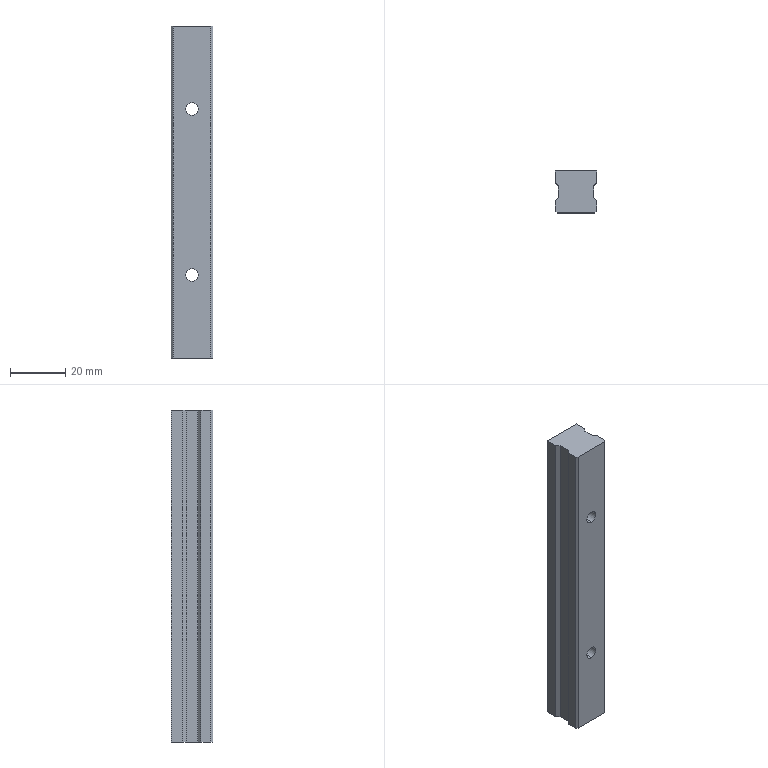Part | SolidWorks | features MoveFace 2, Chamfer 1, Extrusion 1, LPattern 1, RevCut 1 | 1 solid | 26 faces | box 15 x 15 x 120 mm | volume 24720 mm3 | plane 18 | cylinder 8 | commonest cylinder face diameters 4.5 x4 7.5 x4
STEP:
#1=CARTESIAN_POINT('',(0.,9.7,-27.75));
#2=VERTEX_POINT('',#1);
#3=CARTESIAN_POINT('',(0.,9.7,-32.25));
#4=VERTEX_POINT('',#3);
#5=CARTESIAN_POINT('',(0.,9.7,-30.));
#6=DIRECTION('',(0.,-1.,0.));
#7=DIRECTION('',(0.,0.,-1.));
#8=AXIS2_PLACEMENT_3D('',#5,#6,#7);
#9=CIRCLE('',#8,2.25);
#10=EDGE_CURVE('',#2,#4,#9,.T.);
#11=ORIENTED_EDGE('',*,*,#10,.F.);
#12=CARTESIAN_POINT('',(0.,0.,-27.75));
#13=VERTEX_POINT('',#12);
#14=CARTESIAN_POINT('',(0.,15.,-27.75));
#15=DIRECTION('',(0.,-1.,0.));
#16=VECTOR('',#15,1000.);
#17=LINE('',#14,#16);
#18=EDGE_CURVE('',#2,#13,#17,.T.);
#19=ORIENTED_EDGE('',*,*,#18,.T.);
#20=CARTESIAN_POINT('',(0.,0.,-32.25));
#21=VERTEX_POINT('',#20);
#22=CARTESIAN_POINT('',(0.,0.,-30.));
#23=DIRECTION('',(0.,-1.,0.));
#24=DIRECTION('',(0.,0.,-1.));
#25=AXIS2_PLACEMENT_3D('',#22,#23,#24);
#26=CIRCLE('',#25,2.25);
#27=EDGE_CURVE('',#13,#21,#26,.T.);
#28=ORIENTED_EDGE('',*,*,#27,.T.);
#29=CARTESIAN_POINT('',(0.,15.,-32.25));
#30=DIRECTION('',(0.,-1.,0.));
#31=VECTOR('',#30,1000.);
#32=LINE('',#29,#31);
#33=EDGE_CURVE('',#4,#21,#32,.T.);
#34=ORIENTED_EDGE('',*,*,#33,.F.);
#35=EDGE_LOOP('',(#11,#19,#28,#34));
#36=FACE_OUTER_BOUND('',#35,.T.);
#37=CARTESIAN_POINT('',(0.,15.,-30.));
#38=DIRECTION('',(0.,-1.,0.));
#39=DIRECTION('',(0.,0.,-1.));
#40=AXIS2_PLACEMENT_3D('',#37,#38,#39);
#41=CYLINDRICAL_SURFACE('',#40,2.25);
#42=ADVANCED_FACE('',(#36),#41,.F.);
#43=CARTESIAN_POINT('',(0.,15.,-26.25));
#44=VERTEX_POINT('',#43);
#45=CARTESIAN_POINT('',(0.,15.,-33.75));
#46=VERTEX_POINT('',#45);
#47=CARTESIAN_POINT('',(0.,15.,-30.));
#48=DIRECTION('',(0.,-1.,0.));
#49=DIRECTION('',(0.,0.,-1.));
#50=AXIS2_PLACEMENT_3D('',#47,#48,#49);
#51=CIRCLE('',#50,3.75);
#52=EDGE_CURVE('',#44,#46,#51,.T.);
#53=ORIENTED_EDGE('',*,*,#52,.F.);
#54=CARTESIAN_POINT('',(0.,9.7,-26.25));
#55=VERTEX_POINT('',#54);
#56=CARTESIAN_POINT('',(0.,15.,-26.25));
#57=DIRECTION('',(0.,-1.,0.));
#58=VECTOR('',#57,1000.);
#59=LINE('',#56,#58);
#60=EDGE_CURVE('',#44,#55,#59,.T.);
#61=ORIENTED_EDGE('',*,*,#60,.T.);
#62=CARTESIAN_POINT('',(0.,9.7,-33.75));
#63=VERTEX_POINT('',#62);
#64=CARTESIAN_POINT('',(0.,9.7,-30.));
#65=DIRECTION('',(0.,-1.,0.));
#66=DIRECTION('',(0.,0.,-1.));
#67=AXIS2_PLACEMENT_3D('',#64,#65,#66);
#68=CIRCLE('',#67,3.75);
#69=EDGE_CURVE('',#55,#63,#68,.T.);
#70=ORIENTED_EDGE('',*,*,#69,.T.);
#71=CARTESIAN_POINT('',(0.,15.,-33.75));
#72=DIRECTION('',(0.,-1.,0.));
#73=VECTOR('',#72,1000.);
#74=LINE('',#71,#73);
#75=EDGE_CURVE('',#46,#63,#74,.T.);
#76=ORIENTED_EDGE('',*,*,#75,.F.);
#77=EDGE_LOOP('',(#53,#61,#70,#76));
#78=FACE_OUTER_BOUND('',#77,.T.);
#79=CARTESIAN_POINT('',(0.,15.,-30.));
#80=DIRECTION('',(0.,-1.,0.));
#81=DIRECTION('',(0.,0.,-1.));
#82=AXIS2_PLACEMENT_3D('',#79,#80,#81);
#83=CYLINDRICAL_SURFACE('',#82,3.75);
#84=ADVANCED_FACE('',(#78),#83,.F.);
#85=CARTESIAN_POINT('',(0.,9.7,32.25));
#86=VERTEX_POINT('',#85);
#87=CARTESIAN_POINT('',(0.,9.7,27.75));
#88=VERTEX_POINT('',#87);
#89=CARTESIAN_POINT('',(0.,9.7,30.));
#90=DIRECTION('',(0.,-1.,0.));
#91=DIRECTION('',(0.,0.,-1.));
#92=AXIS2_PLACEMENT_3D('',#89,#90,#91);
#93=CIRCLE('',#92,2.25);
#94=EDGE_CURVE('',#86,#88,#93,.T.);
#95=ORIENTED_EDGE('',*,*,#94,.F.);
#96=CARTESIAN_POINT('',(0.,0.,32.25));
#97=VERTEX_POINT('',#96);
#98=CARTESIAN_POINT('',(0.,15.,32.25));
#99=DIRECTION('',(0.,-1.,0.));
#100=VECTOR('',#99,1000.);
#101=LINE('',#98,#100);
#102=EDGE_CURVE('',#86,#97,#101,.T.);
#103=ORIENTED_EDGE('',*,*,#102,.T.);
#104=CARTESIAN_POINT('',(0.,0.,27.75));
#105=VERTEX_POINT('',#104);
#106=CARTESIAN_POINT('',(0.,0.,30.));
#107=DIRECTION('',(0.,-1.,0.));
#108=DIRECTION('',(0.,0.,-1.));
#109=AXIS2_PLACEMENT_3D('',#106,#107,#108);
#110=CIRCLE('',#109,2.25);
#111=EDGE_CURVE('',#97,#105,#110,.T.);
#112=ORIENTED_EDGE('',*,*,#111,.T.);
#113=CARTESIAN_POINT('',(0.,15.,27.75));
#114=DIRECTION('',(0.,-1.,0.));
#115=VECTOR('',#114,1000.);
#116=LINE('',#113,#115);
#117=EDGE_CURVE('',#88,#105,#116,.T.);
#118=ORIENTED_EDGE('',*,*,#117,.F.);
#119=EDGE_LOOP('',(#95,#103,#112,#118));
#120=FACE_OUTER_BOUND('',#119,.T.);
#121=CARTESIAN_POINT('',(0.,15.,30.));
#122=DIRECTION('',(0.,-1.,0.));
#123=DIRECTION('',(0.,0.,-1.));
#124=AXIS2_PLACEMENT_3D('',#121,#122,#123);
#125=CYLINDRICAL_SURFACE('',#124,2.25);
#126=ADVANCED_FACE('',(#120),#125,.F.);
#127=CARTESIAN_POINT('',(0.,15.,33.75));
#128=VERTEX_POINT('',#127);
#129=CARTESIAN_POINT('',(0.,15.,26.25));
#130=VERTEX_POINT('',#129);
#131=CARTESIAN_POINT('',(0.,15.,30.));
#132=DIRECTION('',(0.,-1.,0.));
#133=DIRECTION('',(0.,0.,-1.));
#134=AXIS2_PLACEMENT_3D('',#131,#132,#133);
#135=CIRCLE('',#134,3.75);
#136=EDGE_CURVE('',#128,#130,#135,.T.);
#137=ORIENTED_EDGE('',*,*,#136,.F.);
#138=CARTESIAN_POINT('',(0.,9.7,33.75));
#139=VERTEX_POINT('',#138);
#140=CARTESIAN_POINT('',(0.,15.,33.75));
#141=DIRECTION('',(0.,-1.,0.));
#142=VECTOR('',#141,1000.);
#143=LINE('',#140,#142);
#144=EDGE_CURVE('',#128,#139,#143,.T.);
#145=ORIENTED_EDGE('',*,*,#144,.T.);
#146=CARTESIAN_POINT('',(0.,9.7,26.25));
#147=VERTEX_POINT('',#146);
#148=CARTESIAN_POINT('',(0.,9.7,30.));
#149=DIRECTION('',(0.,-1.,0.));
#150=DIRECTION('',(0.,0.,-1.));
#151=AXIS2_PLACEMENT_3D('',#148,#149,#150);
#152=CIRCLE('',#151,3.75);
#153=EDGE_CURVE('',#139,#147,#152,.T.);
#154=ORIENTED_EDGE('',*,*,#153,.T.);
#155=CARTESIAN_POINT('',(0.,15.,26.25));
#156=DIRECTION('',(0.,-1.,0.));
#157=VECTOR('',#156,1000.);
#158=LINE('',#155,#157);
#159=EDGE_CURVE('',#130,#147,#158,.T.);
#160=ORIENTED_EDGE('',*,*,#159,.F.);
#161=EDGE_LOOP('',(#137,#145,#154,#160));
#162=FACE_OUTER_BOUND('',#161,.T.);
#163=CARTESIAN_POINT('',(0.,15.,30.));
#164=DIRECTION('',(0.,-1.,0.));
#165=DIRECTION('',(0.,0.,-1.));
#166=AXIS2_PLACEMENT_3D('',#163,#164,#165);
#167=CYLINDRICAL_SURFACE('',#166,3.75);
#168=ADVANCED_FACE('',(#162),#167,.F.);
#169=CARTESIAN_POINT('',(-7.5,4.3,-60.));
#170=VERTEX_POINT('',#169);
#171=CARTESIAN_POINT('',(-7.5,0.7,-60.));
#172=VERTEX_POINT('',#171);
#173=CARTESIAN_POINT('',(-7.5,0.,-60.));
#174=DIRECTION('',(0.,-1.,0.));
#175=VECTOR('',#174,1000.);
#176=LINE('',#173,#175);
#177=EDGE_CURVE('',#170,#172,#176,.T.);
#178=ORIENTED_EDGE('',*,*,#177,.T.);
#179=CARTESIAN_POINT('',(-7.5,0.7,60.));
#180=VERTEX_POINT('',#179);
#181=CARTESIAN_POINT('',(-7.5,0.7,50.));
#182=DIRECTION('',(0.,0.,1.));
#183=VECTOR('',#182,1000.);
#184=LINE('',#181,#183);
#185=EDGE_CURVE('',#172,#180,#184,.T.);
#186=ORIENTED_EDGE('',*,*,#185,.T.);
#187=CARTESIAN_POINT('',(-7.5,4.3,60.));
#188=VERTEX_POINT('',#187);
#189=CARTESIAN_POINT('',(-7.5,0.,60.));
#190=DIRECTION('',(0.,-1.,0.));
#191=VECTOR('',#190,1000.);
#192=LINE('',#189,#191);
#193=EDGE_CURVE('',#188,#180,#192,.T.);
#194=ORIENTED_EDGE('',*,*,#193,.F.);
#195=CARTESIAN_POINT('',(-7.5,4.3,50.));
#196=DIRECTION('',(0.,0.,-1.));
#197=VECTOR('',#196,1000.);
#198=LINE('',#195,#197);
#199=EDGE_CURVE('',#188,#170,#198,.T.);
#200=ORIENTED_EDGE('',*,*,#199,.T.);
#201=EDGE_LOOP('',(#178,#186,#194,#200));
#202=FACE_OUTER_BOUND('',#201,.T.);
#203=CARTESIAN_POINT('',(-7.5,0.,50.));
#204=DIRECTION('',(1.,0.,0.));
#205=DIRECTION('',(0.,0.,-1.));
#206=AXIS2_PLACEMENT_3D('',#203,#204,#205);
#207=PLANE('',#206);
#208=ADVANCED_FACE('',(#202),#207,.F.);
#209=CARTESIAN_POINT('',(0.,0.,-30.));
#210=DIRECTION('',(0.,-1.,0.));
#211=DIRECTION('',(0.,0.,-1.));
#212=AXIS2_PLACEMENT_3D('',#209,#210,#211);
#213=CIRCLE('',#212,2.25);
#214=EDGE_CURVE('',#21,#13,#213,.T.);
#215=ORIENTED_EDGE('',*,*,#214,.F.);
#216=ORIENTED_EDGE('',*,*,#27,.F.);
#217=EDGE_LOOP('',(#215,#216));
#218=FACE_BOUND('',#217,.T.);
#219=CARTESIAN_POINT('',(0.,0.,30.));
#220=DIRECTION('',(0.,-1.,0.));
#221=DIRECTION('',(0.,0.,-1.));
#222=AXIS2_PLACEMENT_3D('',#219,#220,#221);
#223=CIRCLE('',#222,2.25);
#224=EDGE_CURVE('',#105,#97,#223,.T.);
#225=ORIENTED_EDGE('',*,*,#224,.F.);
#226=ORIENTED_EDGE('',*,*,#111,.F.);
#227=EDGE_LOOP('',(#225,#226));
#228=FACE_BOUND('',#227,.T.);
#229=CARTESIAN_POINT('',(-6.8,0.,-60.));
#230=VERTEX_POINT('',#229);
#231=CARTESIAN_POINT('',(6.8,0.,-60.));
#232=VERTEX_POINT('',#231);
#233=CARTESIAN_POINT('',(-7.5,0.,-60.));
#234=DIRECTION('',(1.,0.,0.));
#235=VECTOR('',#234,1000.);
#236=LINE('',#233,#235);
#237=EDGE_CURVE('',#230,#232,#236,.T.);
#238=ORIENTED_EDGE('',*,*,#237,.T.);
#239=CARTESIAN_POINT('',(6.8,0.,60.));
#240=VERTEX_POINT('',#239);
#241=CARTESIAN_POINT('',(6.8,0.,50.));
#242=DIRECTION('',(0.,0.,1.));
#243=VECTOR('',#242,1000.);
#244=LINE('',#241,#243);
#245=EDGE_CURVE('',#232,#240,#244,.T.);
#246=ORIENTED_EDGE('',*,*,#245,.T.);
#247=CARTESIAN_POINT('',(-6.8,0.,60.));
#248=VERTEX_POINT('',#247);
#249=CARTESIAN_POINT('',(-7.5,0.,60.));
#250=DIRECTION('',(1.,0.,0.));
#251=VECTOR('',#250,1000.);
#252=LINE('',#249,#251);
#253=EDGE_CURVE('',#248,#240,#252,.T.);
#254=ORIENTED_EDGE('',*,*,#253,.F.);
#255=CARTESIAN_POINT('',(-6.8,0.,50.));
#256=DIRECTION('',(0.,0.,-1.));
#257=VECTOR('',#256,1000.);
#258=LINE('',#255,#257);
#259=EDGE_CURVE('',#248,#230,#258,.T.);
#260=ORIENTED_EDGE('',*,*,#259,.T.);
#261=EDGE_LOOP('',(#238,#246,#254,#260));
#262=FACE_OUTER_BOUND('',#261,.T.);
#263=CARTESIAN_POINT('',(-7.5,0.,50.));
#264=DIRECTION('',(0.,1.,0.));
#265=DIRECTION('',(-1.,0.,0.));
#266=AXIS2_PLACEMENT_3D('',#263,#264,#265);
#267=PLANE('',#266);
#268=ADVANCED_FACE('',(#218,#228,#262),#267,.F.);
#269=CARTESIAN_POINT('',(7.5,0.7,60.));
#270=VERTEX_POINT('',#269);
#271=CARTESIAN_POINT('',(7.5,4.3,60.));
#272=VERTEX_POINT('',#271);
#273=CARTESIAN_POINT('',(7.5,0.,60.));
#274=DIRECTION('',(0.,1.,0.));
#275=VECTOR('',#274,1000.);
#276=LINE('',#273,#275);
#277=EDGE_CURVE('',#270,#272,#276,.T.);
#278=ORIENTED_EDGE('',*,*,#277,.F.);
#279=CARTESIAN_POINT('',(7.5,0.7,-60.));
#280=VERTEX_POINT('',#279);
#281=CARTESIAN_POINT('',(7.5,0.7,50.));
#282=DIRECTION('',(0.,0.,-1.));
#283=VECTOR('',#282,1000.);
#284=LINE('',#281,#283);
#285=EDGE_CURVE('',#270,#280,#284,.T.);
#286=ORIENTED_EDGE('',*,*,#285,.T.);
#287=CARTESIAN_POINT('',(7.5,4.3,-60.));
#288=VERTEX_POINT('',#287);
#289=CARTESIAN_POINT('',(7.5,0.,-60.));
#290=DIRECTION('',(0.,1.,0.));
#291=VECTOR('',#290,1000.);
#292=LINE('',#289,#291);
#293=EDGE_CURVE('',#280,#288,#292,.T.);
#294=ORIENTED_EDGE('',*,*,#293,.T.);
#295=CARTESIAN_POINT('',(7.5,4.3,50.));
#296=DIRECTION('',(0.,0.,-1.));
#297=VECTOR('',#296,1000.);
#298=LINE('',#295,#297);
#299=EDGE_CURVE('',#272,#288,#298,.T.);
#300=ORIENTED_EDGE('',*,*,#299,.F.);
#301=EDGE_LOOP('',(#278,#286,#294,#300));
#302=FACE_OUTER_BOUND('',#301,.T.);
#303=CARTESIAN_POINT('',(7.5,0.,50.));
#304=DIRECTION('',(-1.,0.,0.));
#305=DIRECTION('',(0.,0.,1.));
#306=AXIS2_PLACEMENT_3D('',#303,#304,#305);
#307=PLANE('',#306);
#308=ADVANCED_FACE('',(#302),#307,.F.);
#309=CARTESIAN_POINT('',(6.375,5.425,-60.));
#310=VERTEX_POINT('',#309);
#311=CARTESIAN_POINT('',(7.5,4.3,-60.));
#312=DIRECTION('',(-0.7071,0.7071,0.));
#313=VECTOR('',#312,1000.);
#314=LINE('',#311,#313);
#315=EDGE_CURVE('',#288,#310,#314,.T.);
#316=ORIENTED_EDGE('',*,*,#315,.T.);
#317=CARTESIAN_POINT('',(6.375,5.425,60.));
#318=VERTEX_POINT('',#317);
#319=CARTESIAN_POINT('',(6.375,5.425,50.));
#320=DIRECTION('',(0.,0.,-1.));
#321=VECTOR('',#320,1000.);
#322=LINE('',#319,#321);
#323=EDGE_CURVE('',#318,#310,#322,.T.);
#324=ORIENTED_EDGE('',*,*,#323,.F.);
#325=CARTESIAN_POINT('',(7.5,4.3,60.));
#326=DIRECTION('',(-0.7071,0.7071,0.));
#327=VECTOR('',#326,1000.);
#328=LINE('',#325,#327);
#329=EDGE_CURVE('',#272,#318,#328,.T.);
#330=ORIENTED_EDGE('',*,*,#329,.F.);
#331=ORIENTED_EDGE('',*,*,#299,.T.);
#332=EDGE_LOOP('',(#316,#324,#330,#331));
#333=FACE_OUTER_BOUND('',#332,.T.);
#334=CARTESIAN_POINT('',(7.5,4.3,50.));
#335=DIRECTION('',(-0.7071,-0.7071,0.));
#336=DIRECTION('',(0.7071,-0.7071,0.));
#337=AXIS2_PLACEMENT_3D('',#334,#335,#336);
#338=PLANE('',#337);
#339=ADVANCED_FACE('',(#333),#338,.F.);
#340=CARTESIAN_POINT('',(6.375,9.65,-60.));
#341=VERTEX_POINT('',#340);
#342=CARTESIAN_POINT('',(6.375,5.425,-60.));
#343=DIRECTION('',(0.,1.,0.));
#344=VECTOR('',#343,1000.);
#345=LINE('',#342,#344);
#346=EDGE_CURVE('',#310,#341,#345,.T.);
#347=ORIENTED_EDGE('',*,*,#346,.T.);
#348=CARTESIAN_POINT('',(6.375,9.65,60.));
#349=VERTEX_POINT('',#348);
#350=CARTESIAN_POINT('',(6.375,9.65,50.));
#351=DIRECTION('',(0.,0.,-1.));
#352=VECTOR('',#351,1000.);
#353=LINE('',#350,#352);
#354=EDGE_CURVE('',#349,#341,#353,.T.);
#355=ORIENTED_EDGE('',*,*,#354,.F.);
#356=CARTESIAN_POINT('',(6.375,5.425,60.));
#357=DIRECTION('',(0.,1.,0.));
#358=VECTOR('',#357,1000.);
#359=LINE('',#356,#358);
#360=EDGE_CURVE('',#318,#349,#359,.T.);
#361=ORIENTED_EDGE('',*,*,#360,.F.);
#362=ORIENTED_EDGE('',*,*,#323,.T.);
#363=EDGE_LOOP('',(#347,#355,#361,#362));
#364=FACE_OUTER_BOUND('',#363,.T.);
#365=CARTESIAN_POINT('',(6.375,5.425,50.));
#366=DIRECTION('',(-1.,0.,0.));
#367=DIRECTION('',(0.,0.,1.));
#368=AXIS2_PLACEMENT_3D('',#365,#366,#367);
#369=PLANE('',#368);
#370=ADVANCED_FACE('',(#364),#369,.F.);
#371=CARTESIAN_POINT('',(7.5,10.775,-60.));
#372=VERTEX_POINT('',#371);
#373=CARTESIAN_POINT('',(6.375,9.65,-60.));
#374=DIRECTION('',(0.7071,0.7071,0.));
#375=VECTOR('',#374,1000.);
#376=LINE('',#373,#375);
#377=EDGE_CURVE('',#341,#372,#376,.T.);
#378=ORIENTED_EDGE('',*,*,#377,.T.);
#379=CARTESIAN_POINT('',(7.5,10.775,60.));
#380=VERTEX_POINT('',#379);
#381=CARTESIAN_POINT('',(7.5,10.775,50.));
#382=DIRECTION('',(0.,0.,-1.));
#383=VECTOR('',#382,1000.);
#384=LINE('',#381,#383);
#385=EDGE_CURVE('',#380,#372,#384,.T.);
#386=ORIENTED_EDGE('',*,*,#385,.F.);
#387=CARTESIAN_POINT('',(6.375,9.65,60.));
#388=DIRECTION('',(0.7071,0.7071,0.));
#389=VECTOR('',#388,1000.);
#390=LINE('',#387,#389);
#391=EDGE_CURVE('',#349,#380,#390,.T.);
#392=ORIENTED_EDGE('',*,*,#391,.F.);
#393=ORIENTED_EDGE('',*,*,#354,.T.);
#394=EDGE_LOOP('',(#378,#386,#392,#393));
#395=FACE_OUTER_BOUND('',#394,.T.);
#396=CARTESIAN_POINT('',(6.375,9.65,50.));
#397=DIRECTION('',(-0.7071,0.7071,0.));
#398=DIRECTION('',(-0.7071,-0.7071,0.));
#399=AXIS2_PLACEMENT_3D('',#396,#397,#398);
#400=PLANE('',#399);
#401=ADVANCED_FACE('',(#395),#400,.F.);
#402=CARTESIAN_POINT('',(7.5,15.,-60.));
#403=VERTEX_POINT('',#402);
#404=CARTESIAN_POINT('',(7.5,10.775,-60.));
#405=DIRECTION('',(0.,1.,0.));
#406=VECTOR('',#405,1000.);
#407=LINE('',#404,#406);
#408=EDGE_CURVE('',#372,#403,#407,.T.);
#409=ORIENTED_EDGE('',*,*,#408,.T.);
#410=CARTESIAN_POINT('',(7.5,15.,60.));
#411=VERTEX_POINT('',#410);
#412=CARTESIAN_POINT('',(7.5,15.,50.));
#413=DIRECTION('',(0.,0.,-1.));
#414=VECTOR('',#413,1000.);
#415=LINE('',#412,#414);
#416=EDGE_CURVE('',#411,#403,#415,.T.);
#417=ORIENTED_EDGE('',*,*,#416,.F.);
#418=CARTESIAN_POINT('',(7.5,10.775,60.));
#419=DIRECTION('',(0.,1.,0.));
#420=VECTOR('',#419,1000.);
#421=LINE('',#418,#420);
#422=EDGE_CURVE('',#380,#411,#421,.T.);
#423=ORIENTED_EDGE('',*,*,#422,.F.);
#424=ORIENTED_EDGE('',*,*,#385,.T.);
#425=EDGE_LOOP('',(#409,#417,#423,#424));
#426=FACE_OUTER_BOUND('',#425,.T.);
#427=CARTESIAN_POINT('',(7.5,10.775,50.));
#428=DIRECTION('',(-1.,0.,0.));
#429=DIRECTION('',(0.,0.,1.));
#430=AXIS2_PLACEMENT_3D('',#427,#428,#429);
#431=PLANE('',#430);
#432=ADVANCED_FACE('',(#426),#431,.F.);
#433=CARTESIAN_POINT('',(0.,15.,-30.));
#434=DIRECTION('',(0.,-1.,0.));
#435=DIRECTION('',(0.,0.,-1.));
#436=AXIS2_PLACEMENT_3D('',#433,#434,#435);
#437=CIRCLE('',#436,3.75);
#438=EDGE_CURVE('',#46,#44,#437,.T.);
#439=ORIENTED_EDGE('',*,*,#438,.T.);
#440=ORIENTED_EDGE('',*,*,#52,.T.);
#441=EDGE_LOOP('',(#439,#440));
#442=FACE_BOUND('',#441,.T.);
#443=CARTESIAN_POINT('',(0.,15.,30.));
#444=DIRECTION('',(0.,-1.,0.));
#445=DIRECTION('',(0.,0.,-1.));
#446=AXIS2_PLACEMENT_3D('',#443,#444,#445);
#447=CIRCLE('',#446,3.75);
#448=EDGE_CURVE('',#130,#128,#447,.T.);
#449=ORIENTED_EDGE('',*,*,#448,.T.);
#450=ORIENTED_EDGE('',*,*,#136,.T.);
#451=EDGE_LOOP('',(#449,#450));
#452=FACE_BOUND('',#451,.T.);
#453=CARTESIAN_POINT('',(-7.5,15.,-60.));
#454=VERTEX_POINT('',#453);
#455=CARTESIAN_POINT('',(-7.5,15.,-60.));
#456=DIRECTION('',(-1.,0.,0.));
#457=VECTOR('',#456,1000.);
#458=LINE('',#455,#457);
#459=EDGE_CURVE('',#403,#454,#458,.T.);
#460=ORIENTED_EDGE('',*,*,#459,.T.);
#461=CARTESIAN_POINT('',(-7.5,15.,60.));
#462=VERTEX_POINT('',#461);
#463=CARTESIAN_POINT('',(-7.5,15.,50.));
#464=DIRECTION('',(0.,0.,-1.));
#465=VECTOR('',#464,1000.);
#466=LINE('',#463,#465);
#467=EDGE_CURVE('',#462,#454,#466,.T.);
#468=ORIENTED_EDGE('',*,*,#467,.F.);
#469=CARTESIAN_POINT('',(-7.5,15.,60.));
#470=DIRECTION('',(-1.,0.,0.));
#471=VECTOR('',#470,1000.);
#472=LINE('',#469,#471);
#473=EDGE_CURVE('',#411,#462,#472,.T.);
#474=ORIENTED_EDGE('',*,*,#473,.F.);
#475=ORIENTED_EDGE('',*,*,#416,.T.);
#476=EDGE_LOOP('',(#460,#468,#474,#475));
#477=FACE_OUTER_BOUND('',#476,.T.);
#478=CARTESIAN_POINT('',(-7.5,15.,50.));
#479=DIRECTION('',(0.,-1.,0.));
#480=DIRECTION('',(0.,0.,-1.));
#481=AXIS2_PLACEMENT_3D('',#478,#479,#480);
#482=PLANE('',#481);
#483=ADVANCED_FACE('',(#442,#452,#477),#482,.F.);
#484=CARTESIAN_POINT('',(-7.5,10.775,-60.));
#485=VERTEX_POINT('',#484);
#486=CARTESIAN_POINT('',(-7.5,10.775,-60.));
#487=DIRECTION('',(0.,-1.,0.));
#488=VECTOR('',#487,1000.);
#489=LINE('',#486,#488);
#490=EDGE_CURVE('',#454,#485,#489,.T.);
#491=ORIENTED_EDGE('',*,*,#490,.T.);
#492=CARTESIAN_POINT('',(-7.5,10.775,60.));
#493=VERTEX_POINT('',#492);
#494=CARTESIAN_POINT('',(-7.5,10.775,50.));
#495=DIRECTION('',(0.,0.,-1.));
#496=VECTOR('',#495,1000.);
#497=LINE('',#494,#496);
#498=EDGE_CURVE('',#493,#485,#497,.T.);
#499=ORIENTED_EDGE('',*,*,#498,.F.);
#500=CARTESIAN_POINT('',(-7.5,10.775,60.));
#501=DIRECTION('',(0.,-1.,0.));
#502=VECTOR('',#501,1000.);
#503=LINE('',#500,#502);
#504=EDGE_CURVE('',#462,#493,#503,.T.);
#505=ORIENTED_EDGE('',*,*,#504,.F.);
#506=ORIENTED_EDGE('',*,*,#467,.T.);
#507=EDGE_LOOP('',(#491,#499,#505,#506));
#508=FACE_OUTER_BOUND('',#507,.T.);
#509=CARTESIAN_POINT('',(-7.5,10.775,50.));
#510=DIRECTION('',(1.,0.,0.));
#511=DIRECTION('',(0.,0.,-1.));
#512=AXIS2_PLACEMENT_3D('',#509,#510,#511);
#513=PLANE('',#512);
#514=ADVANCED_FACE('',(#508),#513,.F.);
#515=CARTESIAN_POINT('',(-6.375,9.65,-60.));
#516=VERTEX_POINT('',#515);
#517=CARTESIAN_POINT('',(-6.375,9.65,-60.));
#518=DIRECTION('',(0.7071,-0.7071,0.));
#519=VECTOR('',#518,1000.);
#520=LINE('',#517,#519);
#521=EDGE_CURVE('',#485,#516,#520,.T.);
#522=ORIENTED_EDGE('',*,*,#521,.T.);
#523=CARTESIAN_POINT('',(-6.375,9.65,60.));
#524=VERTEX_POINT('',#523);
#525=CARTESIAN_POINT('',(-6.375,9.65,50.));
#526=DIRECTION('',(0.,0.,-1.));
#527=VECTOR('',#526,1000.);
#528=LINE('',#525,#527);
#529=EDGE_CURVE('',#524,#516,#528,.T.);
#530=ORIENTED_EDGE('',*,*,#529,.F.);
#531=CARTESIAN_POINT('',(-6.375,9.65,60.));
#532=DIRECTION('',(0.7071,-0.7071,0.));
#533=VECTOR('',#532,1000.);
#534=LINE('',#531,#533);
#535=EDGE_CURVE('',#493,#524,#534,.T.);
#536=ORIENTED_EDGE('',*,*,#535,.F.);
#537=ORIENTED_EDGE('',*,*,#498,.T.);
#538=EDGE_LOOP('',(#522,#530,#536,#537));
#539=FACE_OUTER_BOUND('',#538,.T.);
#540=CARTESIAN_POINT('',(-6.375,9.65,50.));
#541=DIRECTION('',(0.7071,0.7071,0.));
#542=DIRECTION('',(-0.7071,0.7071,0.));
#543=AXIS2_PLACEMENT_3D('',#540,#541,#542);
#544=PLANE('',#543);
#545=ADVANCED_FACE('',(#539),#544,.F.);
#546=CARTESIAN_POINT('',(-6.375,5.425,-60.));
#547=VERTEX_POINT('',#546);
#548=CARTESIAN_POINT('',(-6.375,5.425,-60.));
#549=DIRECTION('',(0.,-1.,0.));
#550=VECTOR('',#549,1000.);
#551=LINE('',#548,#550);
#552=EDGE_CURVE('',#516,#547,#551,.T.);
#553=ORIENTED_EDGE('',*,*,#552,.T.);
#554=CARTESIAN_POINT('',(-6.375,5.425,60.));
#555=VERTEX_POINT('',#554);
#556=CARTESIAN_POINT('',(-6.375,5.425,50.));
#557=DIRECTION('',(0.,0.,-1.));
#558=VECTOR('',#557,1000.);
#559=LINE('',#556,#558);
#560=EDGE_CURVE('',#555,#547,#559,.T.);
#561=ORIENTED_EDGE('',*,*,#560,.F.);
#562=CARTESIAN_POINT('',(-6.375,5.425,60.));
#563=DIRECTION('',(0.,-1.,0.));
#564=VECTOR('',#563,1000.);
#565=LINE('',#562,#564);
#566=EDGE_CURVE('',#524,#555,#565,.T.);
#567=ORIENTED_EDGE('',*,*,#566,.F.);
#568=ORIENTED_EDGE('',*,*,#529,.T.);
#569=EDGE_LOOP('',(#553,#561,#567,#568));
#570=FACE_OUTER_BOUND('',#569,.T.);
#571=CARTESIAN_POINT('',(-6.375,5.425,50.));
#572=DIRECTION('',(1.,0.,0.));
#573=DIRECTION('',(0.,0.,-1.));
#574=AXIS2_PLACEMENT_3D('',#571,#572,#573);
#575=PLANE('',#574);
#576=ADVANCED_FACE('',(#570),#575,.F.);
#577=CARTESIAN_POINT('',(-7.5,4.3,-60.));
#578=DIRECTION('',(-0.7071,-0.7071,0.));
#579=VECTOR('',#578,1000.);
#580=LINE('',#577,#579);
#581=EDGE_CURVE('',#547,#170,#580,.T.);
#582=ORIENTED_EDGE('',*,*,#581,.T.);
#583=ORIENTED_EDGE('',*,*,#199,.F.);
#584=CARTESIAN_POINT('',(-7.5,4.3,60.));
#585=DIRECTION('',(-0.7071,-0.7071,0.));
#586=VECTOR('',#585,1000.);
#587=LINE('',#584,#586);
#588=EDGE_CURVE('',#555,#188,#587,.T.);
#589=ORIENTED_EDGE('',*,*,#588,.F.);
#590=ORIENTED_EDGE('',*,*,#560,.T.);
#591=EDGE_LOOP('',(#582,#583,#589,#590));
#592=FACE_OUTER_BOUND('',#591,.T.);
#593=CARTESIAN_POINT('',(-7.5,4.3,50.));
#594=DIRECTION('',(0.7071,-0.7071,0.));
#595=DIRECTION('',(0.7071,0.7071,0.));
#596=AXIS2_PLACEMENT_3D('',#593,#594,#595);
#597=PLANE('',#596);
#598=ADVANCED_FACE('',(#592),#597,.F.);
#599=ORIENTED_EDGE('',*,*,#253,.T.);
#600=CARTESIAN_POINT('',(7.5,0.7,60.));
#601=DIRECTION('',(0.7071,0.7071,0.));
#602=VECTOR('',#601,1000.);
#603=LINE('',#600,#602);
#604=EDGE_CURVE('',#240,#270,#603,.T.);
#605=ORIENTED_EDGE('',*,*,#604,.T.);
#606=ORIENTED_EDGE('',*,*,#277,.T.);
#607=ORIENTED_EDGE('',*,*,#329,.T.);
#608=ORIENTED_EDGE('',*,*,#360,.T.);
#609=ORIENTED_EDGE('',*,*,#391,.T.);
#610=ORIENTED_EDGE('',*,*,#422,.T.);
#611=ORIENTED_EDGE('',*,*,#473,.T.);
#612=ORIENTED_EDGE('',*,*,#504,.T.);
#613=ORIENTED_EDGE('',*,*,#535,.T.);
#614=ORIENTED_EDGE('',*,*,#566,.T.);
#615=ORIENTED_EDGE('',*,*,#588,.T.);
#616=ORIENTED_EDGE('',*,*,#193,.T.);
#617=CARTESIAN_POINT('',(-6.8,0.,60.));
#618=DIRECTION('',(0.7071,-0.7071,0.));
#619=VECTOR('',#618,1000.);
#620=LINE('',#617,#619);
#621=EDGE_CURVE('',#180,#248,#620,.T.);
#622=ORIENTED_EDGE('',*,*,#621,.T.);
#623=EDGE_LOOP('',(#599,#605,#606,#607,#608,#609,#610,#611,#612,#613,#614,#615,#616,#622));
#624=FACE_OUTER_BOUND('',#623,.T.);
#625=CARTESIAN_POINT('',(0.,0.,60.));
#626=DIRECTION('',(0.,0.,-1.));
#627=DIRECTION('',(-1.,0.,0.));
#628=AXIS2_PLACEMENT_3D('',#625,#626,#627);
#629=PLANE('',#628);
#630=ADVANCED_FACE('',(#624),#629,.F.);
#631=ORIENTED_EDGE('',*,*,#293,.F.);
#632=CARTESIAN_POINT('',(3.4,-3.4,-60.));
#633=DIRECTION('',(-0.7071,-0.7071,0.));
#634=VECTOR('',#633,1000.);
#635=LINE('',#632,#634);
#636=EDGE_CURVE('',#280,#232,#635,.T.);
#637=ORIENTED_EDGE('',*,*,#636,.T.);
#638=ORIENTED_EDGE('',*,*,#237,.F.);
#639=CARTESIAN_POINT('',(-3.4,-3.4,-60.));
#640=DIRECTION('',(-0.7071,0.7071,0.));
#641=VECTOR('',#640,1000.);
#642=LINE('',#639,#641);
#643=EDGE_CURVE('',#230,#172,#642,.T.);
#644=ORIENTED_EDGE('',*,*,#643,.T.);
#645=ORIENTED_EDGE('',*,*,#177,.F.);
#646=ORIENTED_EDGE('',*,*,#581,.F.);
#647=ORIENTED_EDGE('',*,*,#552,.F.);
#648=ORIENTED_EDGE('',*,*,#521,.F.);
#649=ORIENTED_EDGE('',*,*,#490,.F.);
#650=ORIENTED_EDGE('',*,*,#459,.F.);
#651=ORIENTED_EDGE('',*,*,#408,.F.);
#652=ORIENTED_EDGE('',*,*,#377,.F.);
#653=ORIENTED_EDGE('',*,*,#346,.F.);
#654=ORIENTED_EDGE('',*,*,#315,.F.);
#655=EDGE_LOOP('',(#631,#637,#638,#644,#645,#646,#647,#648,#649,#650,#651,#652,#653,#654));
#656=FACE_OUTER_BOUND('',#655,.T.);
#657=CARTESIAN_POINT('',(0.,0.,-60.));
#658=DIRECTION('',(0.,0.,-1.));
#659=DIRECTION('',(-1.,0.,0.));
#660=AXIS2_PLACEMENT_3D('',#657,#658,#659);
#661=PLANE('',#660);
#662=ADVANCED_FACE('',(#656),#661,.T.);
#663=ORIENTED_EDGE('',*,*,#604,.F.);
#664=ORIENTED_EDGE('',*,*,#245,.F.);
#665=ORIENTED_EDGE('',*,*,#636,.F.);
#666=ORIENTED_EDGE('',*,*,#285,.F.);
#667=EDGE_LOOP('',(#663,#664,#665,#666));
#668=FACE_OUTER_BOUND('',#667,.T.);
#669=CARTESIAN_POINT('',(7.5,0.7,50.));
#670=DIRECTION('',(-0.7071,0.7071,0.));
#671=DIRECTION('',(0.,0.,-1.));
#672=AXIS2_PLACEMENT_3D('',#669,#670,#671);
#673=PLANE('',#672);
#674=ADVANCED_FACE('',(#668),#673,.F.);
#675=ORIENTED_EDGE('',*,*,#621,.F.);
#676=ORIENTED_EDGE('',*,*,#185,.F.);
#677=ORIENTED_EDGE('',*,*,#643,.F.);
#678=ORIENTED_EDGE('',*,*,#259,.F.);
#679=EDGE_LOOP('',(#675,#676,#677,#678));
#680=FACE_OUTER_BOUND('',#679,.T.);
#681=CARTESIAN_POINT('',(-6.8,0.,50.));
#682=DIRECTION('',(0.7071,0.7071,0.));
#683=DIRECTION('',(0.,0.,-1.));
#684=AXIS2_PLACEMENT_3D('',#681,#682,#683);
#685=PLANE('',#684);
#686=ADVANCED_FACE('',(#680),#685,.F.);
#687=ORIENTED_EDGE('',*,*,#144,.F.);
#688=ORIENTED_EDGE('',*,*,#448,.F.);
#689=ORIENTED_EDGE('',*,*,#159,.T.);
#690=CARTESIAN_POINT('',(0.,9.7,30.));
#691=DIRECTION('',(0.,-1.,0.));
#692=DIRECTION('',(0.,0.,-1.));
#693=AXIS2_PLACEMENT_3D('',#690,#691,#692);
#694=CIRCLE('',#693,3.75);
#695=EDGE_CURVE('',#147,#139,#694,.T.);
#696=ORIENTED_EDGE('',*,*,#695,.T.);
#697=EDGE_LOOP('',(#687,#688,#689,#696));
#698=FACE_OUTER_BOUND('',#697,.T.);
#699=CARTESIAN_POINT('',(0.,15.,30.));
#700=DIRECTION('',(0.,-1.,0.));
#701=DIRECTION('',(0.,0.,-1.));
#702=AXIS2_PLACEMENT_3D('',#699,#700,#701);
#703=CYLINDRICAL_SURFACE('',#702,3.75);
#704=ADVANCED_FACE('',(#698),#703,.F.);
#705=CARTESIAN_POINT('',(0.,9.7,30.));
#706=DIRECTION('',(0.,-1.,0.));
#707=DIRECTION('',(0.,0.,-1.));
#708=AXIS2_PLACEMENT_3D('',#705,#706,#707);
#709=CIRCLE('',#708,2.25);
#710=EDGE_CURVE('',#88,#86,#709,.T.);
#711=ORIENTED_EDGE('',*,*,#710,.T.);
#712=ORIENTED_EDGE('',*,*,#94,.T.);
#713=EDGE_LOOP('',(#711,#712));
#714=FACE_BOUND('',#713,.T.);
#715=ORIENTED_EDGE('',*,*,#695,.F.);
#716=ORIENTED_EDGE('',*,*,#153,.F.);
#717=EDGE_LOOP('',(#715,#716));
#718=FACE_OUTER_BOUND('',#717,.T.);
#719=CARTESIAN_POINT('',(0.,9.7,33.75));
#720=DIRECTION('',(0.,1.,0.));
#721=DIRECTION('',(0.,0.,1.));
#722=AXIS2_PLACEMENT_3D('',#719,#720,#721);
#723=PLANE('',#722);
#724=ADVANCED_FACE('',(#714,#718),#723,.T.);
#725=ORIENTED_EDGE('',*,*,#102,.F.);
#726=ORIENTED_EDGE('',*,*,#710,.F.);
#727=ORIENTED_EDGE('',*,*,#117,.T.);
#728=ORIENTED_EDGE('',*,*,#224,.T.);
#729=EDGE_LOOP('',(#725,#726,#727,#728));
#730=FACE_OUTER_BOUND('',#729,.T.);
#731=CARTESIAN_POINT('',(0.,15.,30.));
#732=DIRECTION('',(0.,-1.,0.));
#733=DIRECTION('',(0.,0.,-1.));
#734=AXIS2_PLACEMENT_3D('',#731,#732,#733);
#735=CYLINDRICAL_SURFACE('',#734,2.25);
#736=ADVANCED_FACE('',(#730),#735,.F.);
#737=ORIENTED_EDGE('',*,*,#60,.F.);
#738=ORIENTED_EDGE('',*,*,#438,.F.);
#739=ORIENTED_EDGE('',*,*,#75,.T.);
#740=CARTESIAN_POINT('',(0.,9.7,-30.));
#741=DIRECTION('',(0.,-1.,0.));
#742=DIRECTION('',(0.,0.,-1.));
#743=AXIS2_PLACEMENT_3D('',#740,#741,#742);
#744=CIRCLE('',#743,3.75);
#745=EDGE_CURVE('',#63,#55,#744,.T.);
#746=ORIENTED_EDGE('',*,*,#745,.T.);
#747=EDGE_LOOP('',(#737,#738,#739,#746));
#748=FACE_OUTER_BOUND('',#747,.T.);
#749=CARTESIAN_POINT('',(0.,15.,-30.));
#750=DIRECTION('',(0.,-1.,0.));
#751=DIRECTION('',(0.,0.,-1.));
#752=AXIS2_PLACEMENT_3D('',#749,#750,#751);
#753=CYLINDRICAL_SURFACE('',#752,3.75);
#754=ADVANCED_FACE('',(#748),#753,.F.);
#755=CARTESIAN_POINT('',(0.,9.7,-30.));
#756=DIRECTION('',(0.,-1.,0.));
#757=DIRECTION('',(0.,0.,-1.));
#758=AXIS2_PLACEMENT_3D('',#755,#756,#757);
#759=CIRCLE('',#758,2.25);
#760=EDGE_CURVE('',#4,#2,#759,.T.);
#761=ORIENTED_EDGE('',*,*,#760,.T.);
#762=ORIENTED_EDGE('',*,*,#10,.T.);
#763=EDGE_LOOP('',(#761,#762));
#764=FACE_BOUND('',#763,.T.);
#765=ORIENTED_EDGE('',*,*,#745,.F.);
#766=ORIENTED_EDGE('',*,*,#69,.F.);
#767=EDGE_LOOP('',(#765,#766));
#768=FACE_OUTER_BOUND('',#767,.T.);
#769=CARTESIAN_POINT('',(0.,9.7,-26.25));
#770=DIRECTION('',(0.,1.,0.));
#771=DIRECTION('',(0.,0.,1.));
#772=AXIS2_PLACEMENT_3D('',#769,#770,#771);
#773=PLANE('',#772);
#774=ADVANCED_FACE('',(#764,#768),#773,.T.);
#775=ORIENTED_EDGE('',*,*,#18,.F.);
#776=ORIENTED_EDGE('',*,*,#760,.F.);
#777=ORIENTED_EDGE('',*,*,#33,.T.);
#778=ORIENTED_EDGE('',*,*,#214,.T.);
#779=EDGE_LOOP('',(#775,#776,#777,#778));
#780=FACE_OUTER_BOUND('',#779,.T.);
#781=CARTESIAN_POINT('',(0.,15.,-30.));
#782=DIRECTION('',(0.,-1.,0.));
#783=DIRECTION('',(0.,0.,-1.));
#784=AXIS2_PLACEMENT_3D('',#781,#782,#783);
#785=CYLINDRICAL_SURFACE('',#784,2.25);
#786=ADVANCED_FACE('',(#780),#785,.F.);
#787=CLOSED_SHELL('',(#42,#84,#126,#168,#208,#268,#308,#339,#370,#401,#432,#483,#514,#545,#576,#598,#630,#662,#674,#686,#704,#724,#736,#754,#774,#786));
#788=MANIFOLD_SOLID_BREP('',#787);
#789=CARTESIAN_POINT('',(0.,0.,0.));
#790=DIRECTION('',(0.,0.,1.));
#791=DIRECTION('',(1.,0.,0.));
#792=AXIS2_PLACEMENT_3D('',#789,#790,#791);
#793=(LENGTH_UNIT()NAMED_UNIT(*)SI_UNIT(.MILLI.,.METRE.));
#794=UNCERTAINTY_MEASURE_WITH_UNIT(LENGTH_MEASURE(0.00001),#793,'','');
#795=(NAMED_UNIT(*)PLANE_ANGLE_UNIT()SI_UNIT($,.RADIAN.));
#796=(NAMED_UNIT(*)SI_UNIT($,.STERADIAN.)SOLID_ANGLE_UNIT());
#797=(GEOMETRIC_REPRESENTATION_CONTEXT(3)GLOBAL_UNCERTAINTY_ASSIGNED_CONTEXT((#794))GLOBAL_UNIT_ASSIGNED_CONTEXT((#793,#795,#796))REPRESENTATION_CONTEXT('',''));
#798=ADVANCED_BREP_SHAPE_REPRESENTATION('',(#788,#792),#797);